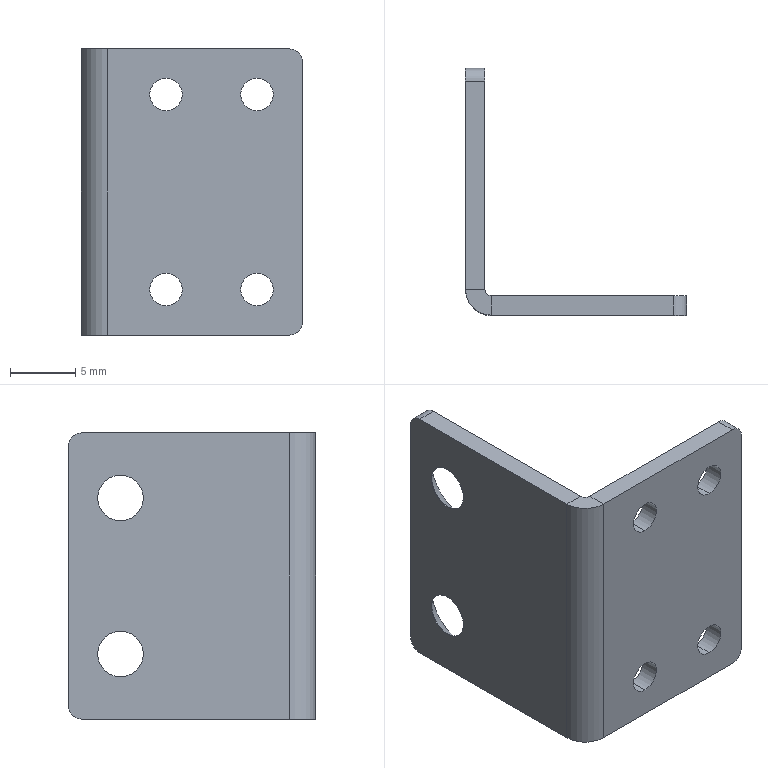Part | NX | features BREP 1 | 1 solid | 34 faces | box 17 x 19 x 22 mm | volume 1032 mm3 | cylinder 18 | plane 12 | cone 4 | commonest cylinder face diameters 2.5 x8 2 x4 3.5 x4 1 x1 4 x1
STEP:
#1=CARTESIAN_POINT('',(-1.45,13.5,7.75));
#2=VERTEX_POINT('',#1);
#3=CARTESIAN_POINT('',(0.,13.5,9.2));
#4=VERTEX_POINT('',#3);
#5=CARTESIAN_POINT('',(0.,13.5,9.2));
#6=DIRECTION('',(0.7071,0.,0.7071));
#7=VECTOR('',#6,1000.);
#8=LINE('',#5,#7);
#9=EDGE_CURVE('',#2,#4,#8,.T.);
#10=ORIENTED_EDGE('',*,*,#9,.F.);
#11=CARTESIAN_POINT('',(-1.45,13.5,4.25));
#12=VERTEX_POINT('',#11);
#13=CARTESIAN_POINT('',(-1.45,13.5,6.));
#14=DIRECTION('',(1.,0.,0.));
#15=DIRECTION('',(0.,0.,-1.));
#16=AXIS2_PLACEMENT_3D('',#13,#14,#15);
#17=CIRCLE('',#16,1.75);
#18=EDGE_CURVE('',#12,#2,#17,.T.);
#19=ORIENTED_EDGE('',*,*,#18,.F.);
#20=CARTESIAN_POINT('',(0.,13.5,2.8));
#21=VERTEX_POINT('',#20);
#22=CARTESIAN_POINT('',(0.,13.5,2.8));
#23=DIRECTION('',(0.7071,0.,-0.7071));
#24=VECTOR('',#23,1000.);
#25=LINE('',#22,#24);
#26=EDGE_CURVE('',#12,#21,#25,.T.);
#27=ORIENTED_EDGE('',*,*,#26,.T.);
#28=CARTESIAN_POINT('',(0.,13.5,6.));
#29=DIRECTION('',(1.,0.,0.));
#30=DIRECTION('',(0.,0.,-1.));
#31=AXIS2_PLACEMENT_3D('',#28,#29,#30);
#32=CIRCLE('',#31,3.2);
#33=EDGE_CURVE('',#21,#4,#32,.T.);
#34=ORIENTED_EDGE('',*,*,#33,.T.);
#35=EDGE_LOOP('',(#10,#19,#27,#34));
#36=FACE_BOUND('',#35,.T.);
#37=CARTESIAN_POINT('',(0.,13.5,6.));
#38=DIRECTION('',(1.,0.,0.));
#39=DIRECTION('',(0.,0.,-1.));
#40=AXIS2_PLACEMENT_3D('',#37,#38,#39);
#41=CONICAL_SURFACE('',#40,3.2,0.7854);
#42=ADVANCED_FACE('',(#36),#41,.F.);
#43=CARTESIAN_POINT('',(-1.5,13.5,7.75));
#44=VERTEX_POINT('',#43);
#45=CARTESIAN_POINT('',(0.,13.5,7.75));
#46=DIRECTION('',(1.,0.,0.));
#47=VECTOR('',#46,1000.);
#48=LINE('',#45,#47);
#49=EDGE_CURVE('',#44,#2,#48,.T.);
#50=ORIENTED_EDGE('',*,*,#49,.F.);
#51=CARTESIAN_POINT('',(-1.5,13.5,4.25));
#52=VERTEX_POINT('',#51);
#53=CARTESIAN_POINT('',(-1.5,13.5,6.));
#54=DIRECTION('',(1.,0.,0.));
#55=DIRECTION('',(0.,0.,-1.));
#56=AXIS2_PLACEMENT_3D('',#53,#54,#55);
#57=CIRCLE('',#56,1.75);
#58=EDGE_CURVE('',#52,#44,#57,.T.);
#59=ORIENTED_EDGE('',*,*,#58,.F.);
#60=CARTESIAN_POINT('',(0.,13.5,4.25));
#61=DIRECTION('',(1.,0.,0.));
#62=VECTOR('',#61,1000.);
#63=LINE('',#60,#62);
#64=EDGE_CURVE('',#52,#12,#63,.T.);
#65=ORIENTED_EDGE('',*,*,#64,.T.);
#66=ORIENTED_EDGE('',*,*,#18,.T.);
#67=EDGE_LOOP('',(#50,#59,#65,#66));
#68=FACE_BOUND('',#67,.T.);
#69=CARTESIAN_POINT('',(0.,13.5,6.));
#70=DIRECTION('',(1.,0.,0.));
#71=DIRECTION('',(0.,0.,-1.));
#72=AXIS2_PLACEMENT_3D('',#69,#70,#71);
#73=CYLINDRICAL_SURFACE('',#72,1.75);
#74=ADVANCED_FACE('',(#68),#73,.F.);
#75=CARTESIAN_POINT('',(-1.45,13.5,-4.25));
#76=VERTEX_POINT('',#75);
#77=CARTESIAN_POINT('',(0.,13.5,-2.8));
#78=VERTEX_POINT('',#77);
#79=CARTESIAN_POINT('',(0.,13.5,-2.8));
#80=DIRECTION('',(0.7071,0.,0.7071));
#81=VECTOR('',#80,1000.);
#82=LINE('',#79,#81);
#83=EDGE_CURVE('',#76,#78,#82,.T.);
#84=ORIENTED_EDGE('',*,*,#83,.F.);
#85=CARTESIAN_POINT('',(-1.45,13.5,-7.75));
#86=VERTEX_POINT('',#85);
#87=CARTESIAN_POINT('',(-1.45,13.5,-6.));
#88=DIRECTION('',(1.,0.,0.));
#89=DIRECTION('',(0.,0.,-1.));
#90=AXIS2_PLACEMENT_3D('',#87,#88,#89);
#91=CIRCLE('',#90,1.75);
#92=EDGE_CURVE('',#86,#76,#91,.T.);
#93=ORIENTED_EDGE('',*,*,#92,.F.);
#94=CARTESIAN_POINT('',(0.,13.5,-9.2));
#95=VERTEX_POINT('',#94);
#96=CARTESIAN_POINT('',(0.,13.5,-9.2));
#97=DIRECTION('',(0.7071,0.,-0.7071));
#98=VECTOR('',#97,1000.);
#99=LINE('',#96,#98);
#100=EDGE_CURVE('',#86,#95,#99,.T.);
#101=ORIENTED_EDGE('',*,*,#100,.T.);
#102=CARTESIAN_POINT('',(0.,13.5,-6.));
#103=DIRECTION('',(1.,0.,0.));
#104=DIRECTION('',(0.,0.,-1.));
#105=AXIS2_PLACEMENT_3D('',#102,#103,#104);
#106=CIRCLE('',#105,3.2);
#107=EDGE_CURVE('',#95,#78,#106,.T.);
#108=ORIENTED_EDGE('',*,*,#107,.T.);
#109=EDGE_LOOP('',(#84,#93,#101,#108));
#110=FACE_BOUND('',#109,.T.);
#111=CARTESIAN_POINT('',(0.,13.5,-6.));
#112=DIRECTION('',(1.,0.,0.));
#113=DIRECTION('',(0.,0.,-1.));
#114=AXIS2_PLACEMENT_3D('',#111,#112,#113);
#115=CONICAL_SURFACE('',#114,3.2,0.7854);
#116=ADVANCED_FACE('',(#110),#115,.F.);
#117=CARTESIAN_POINT('',(-1.5,13.5,-4.25));
#118=VERTEX_POINT('',#117);
#119=CARTESIAN_POINT('',(0.,13.5,-4.25));
#120=DIRECTION('',(1.,0.,0.));
#121=VECTOR('',#120,1000.);
#122=LINE('',#119,#121);
#123=EDGE_CURVE('',#118,#76,#122,.T.);
#124=ORIENTED_EDGE('',*,*,#123,.F.);
#125=CARTESIAN_POINT('',(-1.5,13.5,-7.75));
#126=VERTEX_POINT('',#125);
#127=CARTESIAN_POINT('',(-1.5,13.5,-6.));
#128=DIRECTION('',(1.,0.,0.));
#129=DIRECTION('',(0.,0.,-1.));
#130=AXIS2_PLACEMENT_3D('',#127,#128,#129);
#131=CIRCLE('',#130,1.75);
#132=EDGE_CURVE('',#126,#118,#131,.T.);
#133=ORIENTED_EDGE('',*,*,#132,.F.);
#134=CARTESIAN_POINT('',(0.,13.5,-7.75));
#135=DIRECTION('',(1.,0.,0.));
#136=VECTOR('',#135,1000.);
#137=LINE('',#134,#136);
#138=EDGE_CURVE('',#126,#86,#137,.T.);
#139=ORIENTED_EDGE('',*,*,#138,.T.);
#140=ORIENTED_EDGE('',*,*,#92,.T.);
#141=EDGE_LOOP('',(#124,#133,#139,#140));
#142=FACE_BOUND('',#141,.T.);
#143=CARTESIAN_POINT('',(0.,13.5,-6.));
#144=DIRECTION('',(1.,0.,0.));
#145=DIRECTION('',(0.,0.,-1.));
#146=AXIS2_PLACEMENT_3D('',#143,#144,#145);
#147=CYLINDRICAL_SURFACE('',#146,1.75);
#148=ADVANCED_FACE('',(#142),#147,.F.);
#149=CARTESIAN_POINT('',(12.,0.,-8.75));
#150=VERTEX_POINT('',#149);
#151=CARTESIAN_POINT('',(12.,-1.5,-8.75));
#152=VERTEX_POINT('',#151);
#153=CARTESIAN_POINT('',(12.,0.,-8.75));
#154=DIRECTION('',(0.,1.,0.));
#155=VECTOR('',#154,1000.);
#156=LINE('',#153,#155);
#157=EDGE_CURVE('',#150,#152,#156,.F.);
#158=ORIENTED_EDGE('',*,*,#157,.T.);
#159=CARTESIAN_POINT('',(12.,-1.5,-6.25));
#160=VERTEX_POINT('',#159);
#161=CARTESIAN_POINT('',(12.,-1.5,-7.5));
#162=DIRECTION('',(0.,1.,0.));
#163=DIRECTION('',(0.,0.,1.));
#164=AXIS2_PLACEMENT_3D('',#161,#162,#163);
#165=CIRCLE('',#164,1.25);
#166=EDGE_CURVE('',#160,#152,#165,.T.);
#167=ORIENTED_EDGE('',*,*,#166,.F.);
#168=CARTESIAN_POINT('',(12.,0.,-6.25));
#169=VERTEX_POINT('',#168);
#170=CARTESIAN_POINT('',(12.,0.,-6.25));
#171=DIRECTION('',(0.,1.,0.));
#172=VECTOR('',#171,1000.);
#173=LINE('',#170,#172);
#174=EDGE_CURVE('',#169,#160,#173,.F.);
#175=ORIENTED_EDGE('',*,*,#174,.F.);
#176=CARTESIAN_POINT('',(12.,0.,-7.5));
#177=DIRECTION('',(0.,1.,0.));
#178=DIRECTION('',(0.,0.,1.));
#179=AXIS2_PLACEMENT_3D('',#176,#177,#178);
#180=CIRCLE('',#179,1.25);
#181=EDGE_CURVE('',#169,#150,#180,.T.);
#182=ORIENTED_EDGE('',*,*,#181,.T.);
#183=EDGE_LOOP('',(#158,#167,#175,#182));
#184=FACE_BOUND('',#183,.T.);
#185=CARTESIAN_POINT('',(12.,0.,-7.5));
#186=DIRECTION('',(0.,1.,0.));
#187=DIRECTION('',(0.,0.,1.));
#188=AXIS2_PLACEMENT_3D('',#185,#186,#187);
#189=CYLINDRICAL_SURFACE('',#188,1.25);
#190=ADVANCED_FACE('',(#184),#189,.F.);
#191=CARTESIAN_POINT('',(5.,0.,-8.75));
#192=VERTEX_POINT('',#191);
#193=CARTESIAN_POINT('',(5.,-1.5,-8.75));
#194=VERTEX_POINT('',#193);
#195=CARTESIAN_POINT('',(5.,0.,-8.75));
#196=DIRECTION('',(0.,1.,0.));
#197=VECTOR('',#196,1000.);
#198=LINE('',#195,#197);
#199=EDGE_CURVE('',#192,#194,#198,.F.);
#200=ORIENTED_EDGE('',*,*,#199,.T.);
#201=CARTESIAN_POINT('',(5.,-1.5,-6.25));
#202=VERTEX_POINT('',#201);
#203=CARTESIAN_POINT('',(5.,-1.5,-7.5));
#204=DIRECTION('',(0.,1.,0.));
#205=DIRECTION('',(0.,0.,1.));
#206=AXIS2_PLACEMENT_3D('',#203,#204,#205);
#207=CIRCLE('',#206,1.25);
#208=EDGE_CURVE('',#202,#194,#207,.T.);
#209=ORIENTED_EDGE('',*,*,#208,.F.);
#210=CARTESIAN_POINT('',(5.,0.,-6.25));
#211=VERTEX_POINT('',#210);
#212=CARTESIAN_POINT('',(5.,0.,-6.25));
#213=DIRECTION('',(0.,1.,0.));
#214=VECTOR('',#213,1000.);
#215=LINE('',#212,#214);
#216=EDGE_CURVE('',#211,#202,#215,.F.);
#217=ORIENTED_EDGE('',*,*,#216,.F.);
#218=CARTESIAN_POINT('',(5.,0.,-7.5));
#219=DIRECTION('',(0.,1.,0.));
#220=DIRECTION('',(0.,0.,1.));
#221=AXIS2_PLACEMENT_3D('',#218,#219,#220);
#222=CIRCLE('',#221,1.25);
#223=EDGE_CURVE('',#211,#192,#222,.T.);
#224=ORIENTED_EDGE('',*,*,#223,.T.);
#225=EDGE_LOOP('',(#200,#209,#217,#224));
#226=FACE_BOUND('',#225,.T.);
#227=CARTESIAN_POINT('',(5.,0.,-7.5));
#228=DIRECTION('',(0.,1.,0.));
#229=DIRECTION('',(0.,0.,1.));
#230=AXIS2_PLACEMENT_3D('',#227,#228,#229);
#231=CYLINDRICAL_SURFACE('',#230,1.25);
#232=ADVANCED_FACE('',(#226),#231,.F.);
#233=CARTESIAN_POINT('',(5.,0.,6.25));
#234=VERTEX_POINT('',#233);
#235=CARTESIAN_POINT('',(5.,-1.5,6.25));
#236=VERTEX_POINT('',#235);
#237=CARTESIAN_POINT('',(5.,0.,6.25));
#238=DIRECTION('',(0.,1.,0.));
#239=VECTOR('',#238,1000.);
#240=LINE('',#237,#239);
#241=EDGE_CURVE('',#234,#236,#240,.F.);
#242=ORIENTED_EDGE('',*,*,#241,.T.);
#243=CARTESIAN_POINT('',(5.,-1.5,8.75));
#244=VERTEX_POINT('',#243);
#245=CARTESIAN_POINT('',(5.,-1.5,7.5));
#246=DIRECTION('',(0.,1.,0.));
#247=DIRECTION('',(0.,0.,1.));
#248=AXIS2_PLACEMENT_3D('',#245,#246,#247);
#249=CIRCLE('',#248,1.25);
#250=EDGE_CURVE('',#244,#236,#249,.T.);
#251=ORIENTED_EDGE('',*,*,#250,.F.);
#252=CARTESIAN_POINT('',(5.,0.,8.75));
#253=VERTEX_POINT('',#252);
#254=CARTESIAN_POINT('',(5.,0.,8.75));
#255=DIRECTION('',(0.,1.,0.));
#256=VECTOR('',#255,1000.);
#257=LINE('',#254,#256);
#258=EDGE_CURVE('',#253,#244,#257,.F.);
#259=ORIENTED_EDGE('',*,*,#258,.F.);
#260=CARTESIAN_POINT('',(5.,0.,7.5));
#261=DIRECTION('',(0.,1.,0.));
#262=DIRECTION('',(0.,0.,1.));
#263=AXIS2_PLACEMENT_3D('',#260,#261,#262);
#264=CIRCLE('',#263,1.25);
#265=EDGE_CURVE('',#253,#234,#264,.T.);
#266=ORIENTED_EDGE('',*,*,#265,.T.);
#267=EDGE_LOOP('',(#242,#251,#259,#266));
#268=FACE_BOUND('',#267,.T.);
#269=CARTESIAN_POINT('',(5.,0.,7.5));
#270=DIRECTION('',(0.,1.,0.));
#271=DIRECTION('',(0.,0.,1.));
#272=AXIS2_PLACEMENT_3D('',#269,#270,#271);
#273=CYLINDRICAL_SURFACE('',#272,1.25);
#274=ADVANCED_FACE('',(#268),#273,.F.);
#275=CARTESIAN_POINT('',(12.,0.,6.25));
#276=VERTEX_POINT('',#275);
#277=CARTESIAN_POINT('',(12.,-1.5,6.25));
#278=VERTEX_POINT('',#277);
#279=CARTESIAN_POINT('',(12.,0.,6.25));
#280=DIRECTION('',(0.,1.,0.));
#281=VECTOR('',#280,1000.);
#282=LINE('',#279,#281);
#283=EDGE_CURVE('',#276,#278,#282,.F.);
#284=ORIENTED_EDGE('',*,*,#283,.T.);
#285=CARTESIAN_POINT('',(12.,-1.5,8.75));
#286=VERTEX_POINT('',#285);
#287=CARTESIAN_POINT('',(12.,-1.5,7.5));
#288=DIRECTION('',(0.,1.,0.));
#289=DIRECTION('',(0.,0.,1.));
#290=AXIS2_PLACEMENT_3D('',#287,#288,#289);
#291=CIRCLE('',#290,1.25);
#292=EDGE_CURVE('',#286,#278,#291,.T.);
#293=ORIENTED_EDGE('',*,*,#292,.F.);
#294=CARTESIAN_POINT('',(12.,0.,8.75));
#295=VERTEX_POINT('',#294);
#296=CARTESIAN_POINT('',(12.,0.,8.75));
#297=DIRECTION('',(0.,1.,0.));
#298=VECTOR('',#297,1000.);
#299=LINE('',#296,#298);
#300=EDGE_CURVE('',#295,#286,#299,.F.);
#301=ORIENTED_EDGE('',*,*,#300,.F.);
#302=CARTESIAN_POINT('',(12.,0.,7.5));
#303=DIRECTION('',(0.,1.,0.));
#304=DIRECTION('',(0.,0.,1.));
#305=AXIS2_PLACEMENT_3D('',#302,#303,#304);
#306=CIRCLE('',#305,1.25);
#307=EDGE_CURVE('',#295,#276,#306,.T.);
#308=ORIENTED_EDGE('',*,*,#307,.T.);
#309=EDGE_LOOP('',(#284,#293,#301,#308));
#310=FACE_BOUND('',#309,.T.);
#311=CARTESIAN_POINT('',(12.,0.,7.5));
#312=DIRECTION('',(0.,1.,0.));
#313=DIRECTION('',(0.,0.,1.));
#314=AXIS2_PLACEMENT_3D('',#311,#312,#313);
#315=CYLINDRICAL_SURFACE('',#314,1.25);
#316=ADVANCED_FACE('',(#310),#315,.F.);
#317=CARTESIAN_POINT('',(-1.5,16.5,11.));
#318=VERTEX_POINT('',#317);
#319=CARTESIAN_POINT('',(-1.5,17.5,10.));
#320=VERTEX_POINT('',#319);
#321=CARTESIAN_POINT('',(-1.5,16.5,10.));
#322=DIRECTION('',(-1.,0.,0.));
#323=DIRECTION('',(0.,1.,0.));
#324=AXIS2_PLACEMENT_3D('',#321,#322,#323);
#325=CIRCLE('',#324,1.);
#326=EDGE_CURVE('',#318,#320,#325,.T.);
#327=ORIENTED_EDGE('',*,*,#326,.F.);
#328=CARTESIAN_POINT('',(0.,16.5,11.));
#329=VERTEX_POINT('',#328);
#330=CARTESIAN_POINT('',(-1.5,16.5,11.));
#331=DIRECTION('',(-1.,0.,0.));
#332=VECTOR('',#331,1000.);
#333=LINE('',#330,#332);
#334=EDGE_CURVE('',#329,#318,#333,.T.);
#335=ORIENTED_EDGE('',*,*,#334,.F.);
#336=CARTESIAN_POINT('',(0.,17.5,10.));
#337=VERTEX_POINT('',#336);
#338=CARTESIAN_POINT('',(0.,16.5,10.));
#339=DIRECTION('',(1.,0.,0.));
#340=DIRECTION('',(0.,1.,0.));
#341=AXIS2_PLACEMENT_3D('',#338,#339,#340);
#342=CIRCLE('',#341,1.);
#343=EDGE_CURVE('',#337,#329,#342,.T.);
#344=ORIENTED_EDGE('',*,*,#343,.F.);
#345=CARTESIAN_POINT('',(0.,17.5,10.));
#346=DIRECTION('',(1.,0.,0.));
#347=VECTOR('',#346,1000.);
#348=LINE('',#345,#347);
#349=EDGE_CURVE('',#320,#337,#348,.T.);
#350=ORIENTED_EDGE('',*,*,#349,.F.);
#351=EDGE_LOOP('',(#327,#335,#344,#350));
#352=FACE_BOUND('',#351,.T.);
#353=CARTESIAN_POINT('',(-1.5,16.5,10.));
#354=DIRECTION('',(-1.,0.,0.));
#355=DIRECTION('',(0.,0.,1.));
#356=AXIS2_PLACEMENT_3D('',#353,#354,#355);
#357=CYLINDRICAL_SURFACE('',#356,1.);
#358=ADVANCED_FACE('',(#352),#357,.T.);
#359=CARTESIAN_POINT('',(-1.5,17.5,-10.));
#360=VERTEX_POINT('',#359);
#361=CARTESIAN_POINT('',(-1.5,16.5,-11.));
#362=VERTEX_POINT('',#361);
#363=CARTESIAN_POINT('',(-1.5,16.5,-10.));
#364=DIRECTION('',(-1.,0.,0.));
#365=DIRECTION('',(0.,1.,0.));
#366=AXIS2_PLACEMENT_3D('',#363,#364,#365);
#367=CIRCLE('',#366,1.);
#368=EDGE_CURVE('',#360,#362,#367,.T.);
#369=ORIENTED_EDGE('',*,*,#368,.F.);
#370=CARTESIAN_POINT('',(0.,17.5,-10.));
#371=VERTEX_POINT('',#370);
#372=CARTESIAN_POINT('',(-1.5,17.5,-10.));
#373=DIRECTION('',(-1.,0.,0.));
#374=VECTOR('',#373,1000.);
#375=LINE('',#372,#374);
#376=EDGE_CURVE('',#371,#360,#375,.T.);
#377=ORIENTED_EDGE('',*,*,#376,.F.);
#378=CARTESIAN_POINT('',(0.,16.5,-11.));
#379=VERTEX_POINT('',#378);
#380=CARTESIAN_POINT('',(0.,16.5,-10.));
#381=DIRECTION('',(1.,0.,0.));
#382=DIRECTION('',(0.,1.,0.));
#383=AXIS2_PLACEMENT_3D('',#380,#381,#382);
#384=CIRCLE('',#383,1.);
#385=EDGE_CURVE('',#379,#371,#384,.T.);
#386=ORIENTED_EDGE('',*,*,#385,.F.);
#387=CARTESIAN_POINT('',(0.5,16.5,-11.));
#388=DIRECTION('',(1.,0.,0.));
#389=VECTOR('',#388,1000.);
#390=LINE('',#387,#389);
#391=EDGE_CURVE('',#362,#379,#390,.T.);
#392=ORIENTED_EDGE('',*,*,#391,.F.);
#393=EDGE_LOOP('',(#369,#377,#386,#392));
#394=FACE_BOUND('',#393,.T.);
#395=CARTESIAN_POINT('',(0.5,16.5,-10.));
#396=DIRECTION('',(1.,0.,0.));
#397=DIRECTION('',(0.,0.,-1.));
#398=AXIS2_PLACEMENT_3D('',#395,#396,#397);
#399=CYLINDRICAL_SURFACE('',#398,1.);
#400=ADVANCED_FACE('',(#394),#399,.T.);
#401=CARTESIAN_POINT('',(14.5,0.,11.));
#402=VERTEX_POINT('',#401);
#403=CARTESIAN_POINT('',(15.5,0.,10.));
#404=VERTEX_POINT('',#403);
#405=CARTESIAN_POINT('',(14.5,0.,10.));
#406=DIRECTION('',(0.,1.,0.));
#407=DIRECTION('',(0.,0.,1.));
#408=AXIS2_PLACEMENT_3D('',#405,#406,#407);
#409=CIRCLE('',#408,1.);
#410=EDGE_CURVE('',#402,#404,#409,.T.);
#411=ORIENTED_EDGE('',*,*,#410,.F.);
#412=CARTESIAN_POINT('',(14.5,-1.5,11.));
#413=VERTEX_POINT('',#412);
#414=CARTESIAN_POINT('',(14.5,0.5,11.));
#415=DIRECTION('',(0.,1.,0.));
#416=VECTOR('',#415,1000.);
#417=LINE('',#414,#416);
#418=EDGE_CURVE('',#413,#402,#417,.T.);
#419=ORIENTED_EDGE('',*,*,#418,.F.);
#420=CARTESIAN_POINT('',(15.5,-1.5,10.));
#421=VERTEX_POINT('',#420);
#422=CARTESIAN_POINT('',(14.5,-1.5,10.));
#423=DIRECTION('',(0.,-1.,0.));
#424=DIRECTION('',(0.,0.,1.));
#425=AXIS2_PLACEMENT_3D('',#422,#423,#424);
#426=CIRCLE('',#425,1.);
#427=EDGE_CURVE('',#421,#413,#426,.T.);
#428=ORIENTED_EDGE('',*,*,#427,.F.);
#429=CARTESIAN_POINT('',(15.5,0.,10.));
#430=DIRECTION('',(0.,-1.,0.));
#431=VECTOR('',#430,1000.);
#432=LINE('',#429,#431);
#433=EDGE_CURVE('',#404,#421,#432,.T.);
#434=ORIENTED_EDGE('',*,*,#433,.F.);
#435=EDGE_LOOP('',(#411,#419,#428,#434));
#436=FACE_BOUND('',#435,.T.);
#437=CARTESIAN_POINT('',(14.5,0.,10.));
#438=DIRECTION('',(0.,-1.,0.));
#439=DIRECTION('',(0.,0.,-1.));
#440=AXIS2_PLACEMENT_3D('',#437,#438,#439);
#441=CYLINDRICAL_SURFACE('',#440,1.);
#442=ADVANCED_FACE('',(#436),#441,.T.);
#443=CARTESIAN_POINT('',(15.5,0.,-10.));
#444=VERTEX_POINT('',#443);
#445=CARTESIAN_POINT('',(14.5,0.,-11.));
#446=VERTEX_POINT('',#445);
#447=CARTESIAN_POINT('',(14.5,0.,-10.));
#448=DIRECTION('',(0.,1.,0.));
#449=DIRECTION('',(0.,0.,1.));
#450=AXIS2_PLACEMENT_3D('',#447,#448,#449);
#451=CIRCLE('',#450,1.);
#452=EDGE_CURVE('',#444,#446,#451,.T.);
#453=ORIENTED_EDGE('',*,*,#452,.F.);
#454=CARTESIAN_POINT('',(15.5,-1.5,-10.));
#455=VERTEX_POINT('',#454);
#456=CARTESIAN_POINT('',(15.5,0.,-10.));
#457=DIRECTION('',(0.,1.,0.));
#458=VECTOR('',#457,1000.);
#459=LINE('',#456,#458);
#460=EDGE_CURVE('',#455,#444,#459,.T.);
#461=ORIENTED_EDGE('',*,*,#460,.F.);
#462=CARTESIAN_POINT('',(14.5,-1.5,-11.));
#463=VERTEX_POINT('',#462);
#464=CARTESIAN_POINT('',(14.5,-1.5,-10.));
#465=DIRECTION('',(0.,-1.,0.));
#466=DIRECTION('',(0.,0.,1.));
#467=AXIS2_PLACEMENT_3D('',#464,#465,#466);
#468=CIRCLE('',#467,1.);
#469=EDGE_CURVE('',#463,#455,#468,.T.);
#470=ORIENTED_EDGE('',*,*,#469,.F.);
#471=CARTESIAN_POINT('',(14.5,0.5,-11.));
#472=DIRECTION('',(0.,-1.,0.));
#473=VECTOR('',#472,1000.);
#474=LINE('',#471,#473);
#475=EDGE_CURVE('',#446,#463,#474,.T.);
#476=ORIENTED_EDGE('',*,*,#475,.F.);
#477=EDGE_LOOP('',(#453,#461,#470,#476));
#478=FACE_BOUND('',#477,.T.);
#479=CARTESIAN_POINT('',(14.5,0.5,-10.));
#480=DIRECTION('',(0.,-1.,0.));
#481=DIRECTION('',(0.,0.,-1.));
#482=AXIS2_PLACEMENT_3D('',#479,#480,#481);
#483=CYLINDRICAL_SURFACE('',#482,1.);
#484=ADVANCED_FACE('',(#478),#483,.T.);
#485=CARTESIAN_POINT('',(0.5,0.,-11.));
#486=VERTEX_POINT('',#485);
#487=CARTESIAN_POINT('',(0.,0.,-11.));
#488=DIRECTION('',(1.,0.,0.));
#489=VECTOR('',#488,1000.);
#490=LINE('',#487,#489);
#491=EDGE_CURVE('',#486,#446,#490,.T.);
#492=ORIENTED_EDGE('',*,*,#491,.T.);
#493=ORIENTED_EDGE('',*,*,#475,.T.);
#494=CARTESIAN_POINT('',(0.5,-1.5,-11.));
#495=VERTEX_POINT('',#494);
#496=CARTESIAN_POINT('',(0.,-1.5,-11.));
#497=DIRECTION('',(1.,0.,0.));
#498=VECTOR('',#497,1000.);
#499=LINE('',#496,#498);
#500=EDGE_CURVE('',#495,#463,#499,.T.);
#501=ORIENTED_EDGE('',*,*,#500,.F.);
#502=CARTESIAN_POINT('',(0.5,-1.5,-11.));
#503=DIRECTION('',(0.,1.,0.));
#504=VECTOR('',#503,1000.);
#505=LINE('',#502,#504);
#506=EDGE_CURVE('',#495,#486,#505,.T.);
#507=ORIENTED_EDGE('',*,*,#506,.T.);
#508=EDGE_LOOP('',(#492,#493,#501,#507));
#509=FACE_BOUND('',#508,.T.);
#510=CARTESIAN_POINT('',(0.5,0.5,-11.));
#511=DIRECTION('',(0.,0.,-1.));
#512=DIRECTION('',(-1.,0.,0.));
#513=AXIS2_PLACEMENT_3D('',#510,#511,#512);
#514=PLANE('',#513);
#515=ADVANCED_FACE('',(#509),#514,.T.);
#516=CARTESIAN_POINT('',(0.,0.5,11.));
#517=VERTEX_POINT('',#516);
#518=CARTESIAN_POINT('',(0.,17.5,11.));
#519=DIRECTION('',(0.,-1.,0.));
#520=VECTOR('',#519,1000.);
#521=LINE('',#518,#520);
#522=EDGE_CURVE('',#329,#517,#521,.T.);
#523=ORIENTED_EDGE('',*,*,#522,.F.);
#524=ORIENTED_EDGE('',*,*,#334,.T.);
#525=CARTESIAN_POINT('',(-1.5,0.5,11.));
#526=VERTEX_POINT('',#525);
#527=CARTESIAN_POINT('',(-1.5,17.5,11.));
#528=DIRECTION('',(0.,-1.,0.));
#529=VECTOR('',#528,1000.);
#530=LINE('',#527,#529);
#531=EDGE_CURVE('',#318,#526,#530,.T.);
#532=ORIENTED_EDGE('',*,*,#531,.T.);
#533=CARTESIAN_POINT('',(-1.5,0.5,11.));
#534=DIRECTION('',(1.,0.,0.));
#535=VECTOR('',#534,1000.);
#536=LINE('',#533,#535);
#537=EDGE_CURVE('',#526,#517,#536,.T.);
#538=ORIENTED_EDGE('',*,*,#537,.T.);
#539=EDGE_LOOP('',(#523,#524,#532,#538));
#540=FACE_BOUND('',#539,.T.);
#541=CARTESIAN_POINT('',(0.5,0.5,11.));
#542=DIRECTION('',(0.,0.,-1.));
#543=DIRECTION('',(-1.,0.,0.));
#544=AXIS2_PLACEMENT_3D('',#541,#542,#543);
#545=PLANE('',#544);
#546=ADVANCED_FACE('',(#540),#545,.F.);
#547=CARTESIAN_POINT('',(-1.5,0.5,-11.));
#548=VERTEX_POINT('',#547);
#549=CARTESIAN_POINT('',(0.5,0.5,-11.));
#550=DIRECTION('',(0.,0.,1.));
#551=DIRECTION('',(1.,0.,0.));
#552=AXIS2_PLACEMENT_3D('',#549,#550,#551);
#553=CIRCLE('',#552,2.);
#554=EDGE_CURVE('',#548,#495,#553,.T.);
#555=ORIENTED_EDGE('',*,*,#554,.T.);
#556=CARTESIAN_POINT('',(0.5,-1.5,11.));
#557=VERTEX_POINT('',#556);
#558=CARTESIAN_POINT('',(0.5,-1.5,11.));
#559=DIRECTION('',(0.,0.,-1.));
#560=VECTOR('',#559,1000.);
#561=LINE('',#558,#560);
#562=EDGE_CURVE('',#557,#495,#561,.T.);
#563=ORIENTED_EDGE('',*,*,#562,.F.);
#564=CARTESIAN_POINT('',(0.5,0.5,11.));
#565=DIRECTION('',(0.,0.,1.));
#566=DIRECTION('',(1.,0.,0.));
#567=AXIS2_PLACEMENT_3D('',#564,#565,#566);
#568=CIRCLE('',#567,2.);
#569=EDGE_CURVE('',#526,#557,#568,.T.);
#570=ORIENTED_EDGE('',*,*,#569,.F.);
#571=CARTESIAN_POINT('',(-1.5,0.5,11.));
#572=DIRECTION('',(0.,0.,-1.));
#573=VECTOR('',#572,1000.);
#574=LINE('',#571,#573);
#575=EDGE_CURVE('',#526,#548,#574,.T.);
#576=ORIENTED_EDGE('',*,*,#575,.T.);
#577=EDGE_LOOP('',(#555,#563,#570,#576));
#578=FACE_BOUND('',#577,.T.);
#579=CARTESIAN_POINT('',(0.5,0.5,11.));
#580=DIRECTION('',(0.,0.,-1.));
#581=DIRECTION('',(-1.,0.,0.));
#582=AXIS2_PLACEMENT_3D('',#579,#580,#581);
#583=CYLINDRICAL_SURFACE('',#582,2.);
#584=ADVANCED_FACE('',(#578),#583,.T.);
#585=CARTESIAN_POINT('',(-1.5,17.5,11.));
#586=DIRECTION('',(0.,0.,-1.));
#587=VECTOR('',#586,1000.);
#588=LINE('',#585,#587);
#589=EDGE_CURVE('',#320,#360,#588,.T.);
#590=ORIENTED_EDGE('',*,*,#589,.T.);
#591=ORIENTED_EDGE('',*,*,#368,.T.);
#592=CARTESIAN_POINT('',(-1.5,17.5,-11.));
#593=DIRECTION('',(0.,-1.,0.));
#594=VECTOR('',#593,1000.);
#595=LINE('',#592,#594);
#596=EDGE_CURVE('',#362,#548,#595,.T.);
#597=ORIENTED_EDGE('',*,*,#596,.T.);
#598=ORIENTED_EDGE('',*,*,#575,.F.);
#599=ORIENTED_EDGE('',*,*,#531,.F.);
#600=ORIENTED_EDGE('',*,*,#326,.T.);
#601=EDGE_LOOP('',(#590,#591,#597,#598,#599,#600));
#602=FACE_BOUND('',#601,.T.);
#603=ORIENTED_EDGE('',*,*,#132,.T.);
#604=CARTESIAN_POINT('',(-1.5,13.5,-6.));
#605=DIRECTION('',(1.,0.,0.));
#606=DIRECTION('',(0.,0.,-1.));
#607=AXIS2_PLACEMENT_3D('',#604,#605,#606);
#608=CIRCLE('',#607,1.75);
#609=EDGE_CURVE('',#118,#126,#608,.T.);
#610=ORIENTED_EDGE('',*,*,#609,.T.);
#611=EDGE_LOOP('',(#603,#610));
#612=FACE_BOUND('',#611,.T.);
#613=ORIENTED_EDGE('',*,*,#58,.T.);
#614=CARTESIAN_POINT('',(-1.5,13.5,6.));
#615=DIRECTION('',(1.,0.,0.));
#616=DIRECTION('',(0.,0.,-1.));
#617=AXIS2_PLACEMENT_3D('',#614,#615,#616);
#618=CIRCLE('',#617,1.75);
#619=EDGE_CURVE('',#44,#52,#618,.T.);
#620=ORIENTED_EDGE('',*,*,#619,.T.);
#621=EDGE_LOOP('',(#613,#620));
#622=FACE_BOUND('',#621,.T.);
#623=CARTESIAN_POINT('',(-1.5,17.5,11.));
#624=DIRECTION('',(1.,0.,0.));
#625=DIRECTION('',(0.,1.,0.));
#626=AXIS2_PLACEMENT_3D('',#623,#624,#625);
#627=PLANE('',#626);
#628=ADVANCED_FACE('',(#602,#612,#622),#627,.F.);
#629=CARTESIAN_POINT('',(0.,17.5,11.));
#630=DIRECTION('',(0.,0.,-1.));
#631=VECTOR('',#630,1000.);
#632=LINE('',#629,#631);
#633=EDGE_CURVE('',#337,#371,#632,.T.);
#634=ORIENTED_EDGE('',*,*,#633,.T.);
#635=ORIENTED_EDGE('',*,*,#376,.T.);
#636=ORIENTED_EDGE('',*,*,#589,.F.);
#637=ORIENTED_EDGE('',*,*,#349,.T.);
#638=EDGE_LOOP('',(#634,#635,#636,#637));
#639=FACE_BOUND('',#638,.T.);
#640=CARTESIAN_POINT('',(-1.5,17.5,11.));
#641=DIRECTION('',(0.,1.,0.));
#642=DIRECTION('',(0.,0.,1.));
#643=AXIS2_PLACEMENT_3D('',#640,#641,#642);
#644=PLANE('',#643);
#645=ADVANCED_FACE('',(#639),#644,.T.);
#646=CARTESIAN_POINT('',(0.,0.5,-11.));
#647=VERTEX_POINT('',#646);
#648=CARTESIAN_POINT('',(0.,17.5,-11.));
#649=DIRECTION('',(0.,-1.,0.));
#650=VECTOR('',#649,1000.);
#651=LINE('',#648,#650);
#652=EDGE_CURVE('',#379,#647,#651,.T.);
#653=ORIENTED_EDGE('',*,*,#652,.F.);
#654=ORIENTED_EDGE('',*,*,#385,.T.);
#655=ORIENTED_EDGE('',*,*,#633,.F.);
#656=ORIENTED_EDGE('',*,*,#343,.T.);
#657=ORIENTED_EDGE('',*,*,#522,.T.);
#658=CARTESIAN_POINT('',(0.,0.5,11.));
#659=DIRECTION('',(0.,0.,-1.));
#660=VECTOR('',#659,1000.);
#661=LINE('',#658,#660);
#662=EDGE_CURVE('',#517,#647,#661,.T.);
#663=ORIENTED_EDGE('',*,*,#662,.T.);
#664=EDGE_LOOP('',(#653,#654,#655,#656,#657,#663));
#665=FACE_BOUND('',#664,.T.);
#666=ORIENTED_EDGE('',*,*,#107,.F.);
#667=CARTESIAN_POINT('',(0.,13.5,-6.));
#668=DIRECTION('',(1.,0.,0.));
#669=DIRECTION('',(0.,0.,-1.));
#670=AXIS2_PLACEMENT_3D('',#667,#668,#669);
#671=CIRCLE('',#670,3.2);
#672=EDGE_CURVE('',#78,#95,#671,.T.);
#673=ORIENTED_EDGE('',*,*,#672,.F.);
#674=EDGE_LOOP('',(#666,#673));
#675=FACE_BOUND('',#674,.T.);
#676=ORIENTED_EDGE('',*,*,#33,.F.);
#677=CARTESIAN_POINT('',(0.,13.5,6.));
#678=DIRECTION('',(1.,0.,0.));
#679=DIRECTION('',(0.,0.,-1.));
#680=AXIS2_PLACEMENT_3D('',#677,#678,#679);
#681=CIRCLE('',#680,3.2);
#682=EDGE_CURVE('',#4,#21,#681,.T.);
#683=ORIENTED_EDGE('',*,*,#682,.F.);
#684=EDGE_LOOP('',(#676,#683));
#685=FACE_BOUND('',#684,.T.);
#686=CARTESIAN_POINT('',(0.,17.5,11.));
#687=DIRECTION('',(1.,0.,0.));
#688=DIRECTION('',(0.,1.,0.));
#689=AXIS2_PLACEMENT_3D('',#686,#687,#688);
#690=PLANE('',#689);
#691=ADVANCED_FACE('',(#665,#675,#685),#690,.T.);
#692=CARTESIAN_POINT('',(0.5,0.5,-11.));
#693=DIRECTION('',(0.,0.,1.));
#694=DIRECTION('',(-1.,0.,0.));
#695=AXIS2_PLACEMENT_3D('',#692,#693,#694);
#696=CIRCLE('',#695,0.5);
#697=EDGE_CURVE('',#647,#486,#696,.T.);
#698=ORIENTED_EDGE('',*,*,#697,.F.);
#699=ORIENTED_EDGE('',*,*,#662,.F.);
#700=CARTESIAN_POINT('',(0.5,0.,11.));
#701=VERTEX_POINT('',#700);
#702=CARTESIAN_POINT('',(0.5,0.5,11.));
#703=DIRECTION('',(0.,0.,1.));
#704=DIRECTION('',(-1.,0.,0.));
#705=AXIS2_PLACEMENT_3D('',#702,#703,#704);
#706=CIRCLE('',#705,0.5);
#707=EDGE_CURVE('',#517,#701,#706,.T.);
#708=ORIENTED_EDGE('',*,*,#707,.T.);
#709=CARTESIAN_POINT('',(0.5,0.,11.));
#710=DIRECTION('',(0.,0.,-1.));
#711=VECTOR('',#710,1000.);
#712=LINE('',#709,#711);
#713=EDGE_CURVE('',#701,#486,#712,.T.);
#714=ORIENTED_EDGE('',*,*,#713,.T.);
#715=EDGE_LOOP('',(#698,#699,#708,#714));
#716=FACE_BOUND('',#715,.T.);
#717=CARTESIAN_POINT('',(0.5,0.5,11.));
#718=DIRECTION('',(0.,0.,-1.));
#719=DIRECTION('',(-1.,0.,0.));
#720=AXIS2_PLACEMENT_3D('',#717,#718,#719);
#721=CYLINDRICAL_SURFACE('',#720,0.5);
#722=ADVANCED_FACE('',(#716),#721,.F.);
#723=CARTESIAN_POINT('',(15.5,0.,11.));
#724=DIRECTION('',(0.,0.,-1.));
#725=VECTOR('',#724,1000.);
#726=LINE('',#723,#725);
#727=EDGE_CURVE('',#404,#444,#726,.T.);
#728=ORIENTED_EDGE('',*,*,#727,.T.);
#729=ORIENTED_EDGE('',*,*,#452,.T.);
#730=ORIENTED_EDGE('',*,*,#491,.F.);
#731=ORIENTED_EDGE('',*,*,#713,.F.);
#732=CARTESIAN_POINT('',(0.,0.,11.));
#733=DIRECTION('',(1.,0.,0.));
#734=VECTOR('',#733,1000.);
#735=LINE('',#732,#734);
#736=EDGE_CURVE('',#701,#402,#735,.T.);
#737=ORIENTED_EDGE('',*,*,#736,.T.);
#738=ORIENTED_EDGE('',*,*,#410,.T.);
#739=EDGE_LOOP('',(#728,#729,#730,#731,#737,#738));
#740=FACE_BOUND('',#739,.T.);
#741=ORIENTED_EDGE('',*,*,#307,.F.);
#742=CARTESIAN_POINT('',(12.,0.,7.5));
#743=DIRECTION('',(0.,1.,0.));
#744=DIRECTION('',(0.,0.,1.));
#745=AXIS2_PLACEMENT_3D('',#742,#743,#744);
#746=CIRCLE('',#745,1.25);
#747=EDGE_CURVE('',#276,#295,#746,.T.);
#748=ORIENTED_EDGE('',*,*,#747,.F.);
#749=EDGE_LOOP('',(#741,#748));
#750=FACE_BOUND('',#749,.T.);
#751=ORIENTED_EDGE('',*,*,#265,.F.);
#752=CARTESIAN_POINT('',(5.,0.,7.5));
#753=DIRECTION('',(0.,1.,0.));
#754=DIRECTION('',(0.,0.,1.));
#755=AXIS2_PLACEMENT_3D('',#752,#753,#754);
#756=CIRCLE('',#755,1.25);
#757=EDGE_CURVE('',#234,#253,#756,.T.);
#758=ORIENTED_EDGE('',*,*,#757,.F.);
#759=EDGE_LOOP('',(#751,#758));
#760=FACE_BOUND('',#759,.T.);
#761=ORIENTED_EDGE('',*,*,#223,.F.);
#762=CARTESIAN_POINT('',(5.,0.,-7.5));
#763=DIRECTION('',(0.,1.,0.));
#764=DIRECTION('',(0.,0.,1.));
#765=AXIS2_PLACEMENT_3D('',#762,#763,#764);
#766=CIRCLE('',#765,1.25);
#767=EDGE_CURVE('',#192,#211,#766,.T.);
#768=ORIENTED_EDGE('',*,*,#767,.F.);
#769=EDGE_LOOP('',(#761,#768));
#770=FACE_BOUND('',#769,.T.);
#771=ORIENTED_EDGE('',*,*,#181,.F.);
#772=CARTESIAN_POINT('',(12.,0.,-7.5));
#773=DIRECTION('',(0.,1.,0.));
#774=DIRECTION('',(0.,0.,1.));
#775=AXIS2_PLACEMENT_3D('',#772,#773,#774);
#776=CIRCLE('',#775,1.25);
#777=EDGE_CURVE('',#150,#169,#776,.T.);
#778=ORIENTED_EDGE('',*,*,#777,.F.);
#779=EDGE_LOOP('',(#771,#778));
#780=FACE_BOUND('',#779,.T.);
#781=CARTESIAN_POINT('',(0.,0.,11.));
#782=DIRECTION('',(0.,1.,0.));
#783=DIRECTION('',(0.,0.,1.));
#784=AXIS2_PLACEMENT_3D('',#781,#782,#783);
#785=PLANE('',#784);
#786=ADVANCED_FACE('',(#740,#750,#760,#770,#780),#785,.T.);
#787=CARTESIAN_POINT('',(15.5,-1.5,11.));
#788=DIRECTION('',(0.,0.,-1.));
#789=VECTOR('',#788,1000.);
#790=LINE('',#787,#789);
#791=EDGE_CURVE('',#421,#455,#790,.T.);
#792=ORIENTED_EDGE('',*,*,#791,.T.);
#793=ORIENTED_EDGE('',*,*,#460,.T.);
#794=ORIENTED_EDGE('',*,*,#727,.F.);
#795=ORIENTED_EDGE('',*,*,#433,.T.);
#796=EDGE_LOOP('',(#792,#793,#794,#795));
#797=FACE_BOUND('',#796,.T.);
#798=CARTESIAN_POINT('',(15.5,0.,11.));
#799=DIRECTION('',(1.,0.,0.));
#800=DIRECTION('',(0.,0.,-1.));
#801=AXIS2_PLACEMENT_3D('',#798,#799,#800);
#802=PLANE('',#801);
#803=ADVANCED_FACE('',(#797),#802,.T.);
#804=ORIENTED_EDGE('',*,*,#500,.T.);
#805=ORIENTED_EDGE('',*,*,#469,.T.);
#806=ORIENTED_EDGE('',*,*,#791,.F.);
#807=ORIENTED_EDGE('',*,*,#427,.T.);
#808=CARTESIAN_POINT('',(0.,-1.5,11.));
#809=DIRECTION('',(1.,0.,0.));
#810=VECTOR('',#809,1000.);
#811=LINE('',#808,#810);
#812=EDGE_CURVE('',#557,#413,#811,.T.);
#813=ORIENTED_EDGE('',*,*,#812,.F.);
#814=ORIENTED_EDGE('',*,*,#562,.T.);
#815=EDGE_LOOP('',(#804,#805,#806,#807,#813,#814));
#816=FACE_BOUND('',#815,.T.);
#817=ORIENTED_EDGE('',*,*,#292,.T.);
#818=CARTESIAN_POINT('',(12.,-1.5,7.5));
#819=DIRECTION('',(0.,1.,0.));
#820=DIRECTION('',(0.,0.,1.));
#821=AXIS2_PLACEMENT_3D('',#818,#819,#820);
#822=CIRCLE('',#821,1.25);
#823=EDGE_CURVE('',#278,#286,#822,.T.);
#824=ORIENTED_EDGE('',*,*,#823,.T.);
#825=EDGE_LOOP('',(#817,#824));
#826=FACE_BOUND('',#825,.T.);
#827=ORIENTED_EDGE('',*,*,#250,.T.);
#828=CARTESIAN_POINT('',(5.,-1.5,7.5));
#829=DIRECTION('',(0.,1.,0.));
#830=DIRECTION('',(0.,0.,1.));
#831=AXIS2_PLACEMENT_3D('',#828,#829,#830);
#832=CIRCLE('',#831,1.25);
#833=EDGE_CURVE('',#236,#244,#832,.T.);
#834=ORIENTED_EDGE('',*,*,#833,.T.);
#835=EDGE_LOOP('',(#827,#834));
#836=FACE_BOUND('',#835,.T.);
#837=ORIENTED_EDGE('',*,*,#208,.T.);
#838=CARTESIAN_POINT('',(5.,-1.5,-7.5));
#839=DIRECTION('',(0.,1.,0.));
#840=DIRECTION('',(0.,0.,1.));
#841=AXIS2_PLACEMENT_3D('',#838,#839,#840);
#842=CIRCLE('',#841,1.25);
#843=EDGE_CURVE('',#194,#202,#842,.T.);
#844=ORIENTED_EDGE('',*,*,#843,.T.);
#845=EDGE_LOOP('',(#837,#844));
#846=FACE_BOUND('',#845,.T.);
#847=ORIENTED_EDGE('',*,*,#166,.T.);
#848=CARTESIAN_POINT('',(12.,-1.5,-7.5));
#849=DIRECTION('',(0.,1.,0.));
#850=DIRECTION('',(0.,0.,1.));
#851=AXIS2_PLACEMENT_3D('',#848,#849,#850);
#852=CIRCLE('',#851,1.25);
#853=EDGE_CURVE('',#152,#160,#852,.T.);
#854=ORIENTED_EDGE('',*,*,#853,.T.);
#855=EDGE_LOOP('',(#847,#854));
#856=FACE_BOUND('',#855,.T.);
#857=CARTESIAN_POINT('',(0.,-1.5,11.));
#858=DIRECTION('',(0.,1.,0.));
#859=DIRECTION('',(0.,0.,1.));
#860=AXIS2_PLACEMENT_3D('',#857,#858,#859);
#861=PLANE('',#860);
#862=ADVANCED_FACE('',(#816,#826,#836,#846,#856),#861,.F.);
#863=ORIENTED_EDGE('',*,*,#596,.F.);
#864=ORIENTED_EDGE('',*,*,#391,.T.);
#865=ORIENTED_EDGE('',*,*,#652,.T.);
#866=CARTESIAN_POINT('',(0.,0.5,-11.));
#867=DIRECTION('',(-1.,0.,0.));
#868=VECTOR('',#867,1000.);
#869=LINE('',#866,#868);
#870=EDGE_CURVE('',#647,#548,#869,.T.);
#871=ORIENTED_EDGE('',*,*,#870,.T.);
#872=EDGE_LOOP('',(#863,#864,#865,#871));
#873=FACE_BOUND('',#872,.T.);
#874=CARTESIAN_POINT('',(0.5,-1.5,-11.));
#875=DIRECTION('',(0.,0.,-1.));
#876=DIRECTION('',(-1.,0.,0.));
#877=AXIS2_PLACEMENT_3D('',#874,#875,#876);
#878=PLANE('',#877);
#879=ADVANCED_FACE('',(#873),#878,.T.);
#880=ORIENTED_EDGE('',*,*,#870,.F.);
#881=ORIENTED_EDGE('',*,*,#697,.T.);
#882=ORIENTED_EDGE('',*,*,#506,.F.);
#883=ORIENTED_EDGE('',*,*,#554,.F.);
#884=EDGE_LOOP('',(#880,#881,#882,#883));
#885=FACE_BOUND('',#884,.T.);
#886=CARTESIAN_POINT('',(0.,0.5,-11.));
#887=DIRECTION('',(0.,0.,-1.));
#888=DIRECTION('',(-1.,0.,0.));
#889=AXIS2_PLACEMENT_3D('',#886,#887,#888);
#890=PLANE('',#889);
#891=ADVANCED_FACE('',(#885),#890,.T.);
#892=ORIENTED_EDGE('',*,*,#812,.T.);
#893=ORIENTED_EDGE('',*,*,#418,.T.);
#894=ORIENTED_EDGE('',*,*,#736,.F.);
#895=CARTESIAN_POINT('',(0.5,0.,11.));
#896=DIRECTION('',(0.,-1.,0.));
#897=VECTOR('',#896,1000.);
#898=LINE('',#895,#897);
#899=EDGE_CURVE('',#701,#557,#898,.T.);
#900=ORIENTED_EDGE('',*,*,#899,.T.);
#901=EDGE_LOOP('',(#892,#893,#894,#900));
#902=FACE_BOUND('',#901,.T.);
#903=CARTESIAN_POINT('',(-1.5,0.5,11.));
#904=DIRECTION('',(0.,0.,1.));
#905=DIRECTION('',(1.,0.,0.));
#906=AXIS2_PLACEMENT_3D('',#903,#904,#905);
#907=PLANE('',#906);
#908=ADVANCED_FACE('',(#902),#907,.T.);
#909=ORIENTED_EDGE('',*,*,#899,.F.);
#910=ORIENTED_EDGE('',*,*,#707,.F.);
#911=ORIENTED_EDGE('',*,*,#537,.F.);
#912=ORIENTED_EDGE('',*,*,#569,.T.);
#913=EDGE_LOOP('',(#909,#910,#911,#912));
#914=FACE_BOUND('',#913,.T.);
#915=CARTESIAN_POINT('',(0.5,0.,11.));
#916=DIRECTION('',(0.,0.,1.));
#917=DIRECTION('',(1.,0.,0.));
#918=AXIS2_PLACEMENT_3D('',#915,#916,#917);
#919=PLANE('',#918);
#920=ADVANCED_FACE('',(#914),#919,.T.);
#921=ORIENTED_EDGE('',*,*,#823,.F.);
#922=ORIENTED_EDGE('',*,*,#283,.F.);
#923=ORIENTED_EDGE('',*,*,#747,.T.);
#924=ORIENTED_EDGE('',*,*,#300,.T.);
#925=EDGE_LOOP('',(#921,#922,#923,#924));
#926=FACE_BOUND('',#925,.T.);
#927=CARTESIAN_POINT('',(12.,0.,7.5));
#928=DIRECTION('',(0.,1.,0.));
#929=DIRECTION('',(0.,0.,1.));
#930=AXIS2_PLACEMENT_3D('',#927,#928,#929);
#931=CYLINDRICAL_SURFACE('',#930,1.25);
#932=ADVANCED_FACE('',(#926),#931,.F.);
#933=ORIENTED_EDGE('',*,*,#833,.F.);
#934=ORIENTED_EDGE('',*,*,#241,.F.);
#935=ORIENTED_EDGE('',*,*,#757,.T.);
#936=ORIENTED_EDGE('',*,*,#258,.T.);
#937=EDGE_LOOP('',(#933,#934,#935,#936));
#938=FACE_BOUND('',#937,.T.);
#939=CARTESIAN_POINT('',(5.,0.,7.5));
#940=DIRECTION('',(0.,1.,0.));
#941=DIRECTION('',(0.,0.,1.));
#942=AXIS2_PLACEMENT_3D('',#939,#940,#941);
#943=CYLINDRICAL_SURFACE('',#942,1.25);
#944=ADVANCED_FACE('',(#938),#943,.F.);
#945=ORIENTED_EDGE('',*,*,#843,.F.);
#946=ORIENTED_EDGE('',*,*,#199,.F.);
#947=ORIENTED_EDGE('',*,*,#767,.T.);
#948=ORIENTED_EDGE('',*,*,#216,.T.);
#949=EDGE_LOOP('',(#945,#946,#947,#948));
#950=FACE_BOUND('',#949,.T.);
#951=CARTESIAN_POINT('',(5.,0.,-7.5));
#952=DIRECTION('',(0.,1.,0.));
#953=DIRECTION('',(0.,0.,1.));
#954=AXIS2_PLACEMENT_3D('',#951,#952,#953);
#955=CYLINDRICAL_SURFACE('',#954,1.25);
#956=ADVANCED_FACE('',(#950),#955,.F.);
#957=ORIENTED_EDGE('',*,*,#853,.F.);
#958=ORIENTED_EDGE('',*,*,#157,.F.);
#959=ORIENTED_EDGE('',*,*,#777,.T.);
#960=ORIENTED_EDGE('',*,*,#174,.T.);
#961=EDGE_LOOP('',(#957,#958,#959,#960));
#962=FACE_BOUND('',#961,.T.);
#963=CARTESIAN_POINT('',(12.,0.,-7.5));
#964=DIRECTION('',(0.,1.,0.));
#965=DIRECTION('',(0.,0.,1.));
#966=AXIS2_PLACEMENT_3D('',#963,#964,#965);
#967=CYLINDRICAL_SURFACE('',#966,1.25);
#968=ADVANCED_FACE('',(#962),#967,.F.);
#969=ORIENTED_EDGE('',*,*,#609,.F.);
#970=ORIENTED_EDGE('',*,*,#123,.T.);
#971=CARTESIAN_POINT('',(-1.45,13.5,-6.));
#972=DIRECTION('',(1.,0.,0.));
#973=DIRECTION('',(0.,0.,-1.));
#974=AXIS2_PLACEMENT_3D('',#971,#972,#973);
#975=CIRCLE('',#974,1.75);
#976=EDGE_CURVE('',#76,#86,#975,.T.);
#977=ORIENTED_EDGE('',*,*,#976,.T.);
#978=ORIENTED_EDGE('',*,*,#138,.F.);
#979=EDGE_LOOP('',(#969,#970,#977,#978));
#980=FACE_BOUND('',#979,.T.);
#981=CARTESIAN_POINT('',(0.,13.5,-6.));
#982=DIRECTION('',(1.,0.,0.));
#983=DIRECTION('',(0.,0.,-1.));
#984=AXIS2_PLACEMENT_3D('',#981,#982,#983);
#985=CYLINDRICAL_SURFACE('',#984,1.75);
#986=ADVANCED_FACE('',(#980),#985,.F.);
#987=ORIENTED_EDGE('',*,*,#976,.F.);
#988=ORIENTED_EDGE('',*,*,#83,.T.);
#989=ORIENTED_EDGE('',*,*,#672,.T.);
#990=ORIENTED_EDGE('',*,*,#100,.F.);
#991=EDGE_LOOP('',(#987,#988,#989,#990));
#992=FACE_BOUND('',#991,.T.);
#993=CARTESIAN_POINT('',(0.,13.5,-6.));
#994=DIRECTION('',(1.,0.,0.));
#995=DIRECTION('',(0.,0.,-1.));
#996=AXIS2_PLACEMENT_3D('',#993,#994,#995);
#997=CONICAL_SURFACE('',#996,3.2,0.7854);
#998=ADVANCED_FACE('',(#992),#997,.F.);
#999=ORIENTED_EDGE('',*,*,#619,.F.);
#1000=ORIENTED_EDGE('',*,*,#49,.T.);
#1001=CARTESIAN_POINT('',(-1.45,13.5,6.));
#1002=DIRECTION('',(1.,0.,0.));
#1003=DIRECTION('',(0.,0.,-1.));
#1004=AXIS2_PLACEMENT_3D('',#1001,#1002,#1003);
#1005=CIRCLE('',#1004,1.75);
#1006=EDGE_CURVE('',#2,#12,#1005,.T.);
#1007=ORIENTED_EDGE('',*,*,#1006,.T.);
#1008=ORIENTED_EDGE('',*,*,#64,.F.);
#1009=EDGE_LOOP('',(#999,#1000,#1007,#1008));
#1010=FACE_BOUND('',#1009,.T.);
#1011=CARTESIAN_POINT('',(0.,13.5,6.));
#1012=DIRECTION('',(1.,0.,0.));
#1013=DIRECTION('',(0.,0.,-1.));
#1014=AXIS2_PLACEMENT_3D('',#1011,#1012,#1013);
#1015=CYLINDRICAL_SURFACE('',#1014,1.75);
#1016=ADVANCED_FACE('',(#1010),#1015,.F.);
#1017=ORIENTED_EDGE('',*,*,#1006,.F.);
#1018=ORIENTED_EDGE('',*,*,#9,.T.);
#1019=ORIENTED_EDGE('',*,*,#682,.T.);
#1020=ORIENTED_EDGE('',*,*,#26,.F.);
#1021=EDGE_LOOP('',(#1017,#1018,#1019,#1020));
#1022=FACE_BOUND('',#1021,.T.);
#1023=CARTESIAN_POINT('',(0.,13.5,6.));
#1024=DIRECTION('',(1.,0.,0.));
#1025=DIRECTION('',(0.,0.,-1.));
#1026=AXIS2_PLACEMENT_3D('',#1023,#1024,#1025);
#1027=CONICAL_SURFACE('',#1026,3.2,0.7854);
#1028=ADVANCED_FACE('',(#1022),#1027,.F.);
#1029=CLOSED_SHELL('',(#42,#74,#116,#148,#190,#232,#274,#316,#358,#400,#442,#484,#515,#546,#584,#628,#645,#691,#722,#786,#803,#862,#879,#891,#908,#920,#932,#944,#956,#968,#986,#998,#1016,#1028));
#1030=MANIFOLD_SOLID_BREP('',#1029);
#1031=(LENGTH_UNIT()NAMED_UNIT(*)SI_UNIT(.MILLI.,.METRE.));
#1032=UNCERTAINTY_MEASURE_WITH_UNIT(LENGTH_MEASURE(0.00001),#1031,'','');
#1033=(NAMED_UNIT(*)PLANE_ANGLE_UNIT()SI_UNIT($,.RADIAN.));
#1034=(NAMED_UNIT(*)SI_UNIT($,.STERADIAN.)SOLID_ANGLE_UNIT());
#1035=(GEOMETRIC_REPRESENTATION_CONTEXT(3)GLOBAL_UNCERTAINTY_ASSIGNED_CONTEXT((#1032))GLOBAL_UNIT_ASSIGNED_CONTEXT((#1031,#1033,#1034))REPRESENTATION_CONTEXT('',''));
#1036=ADVANCED_BREP_SHAPE_REPRESENTATION('',(#1030),#1035);